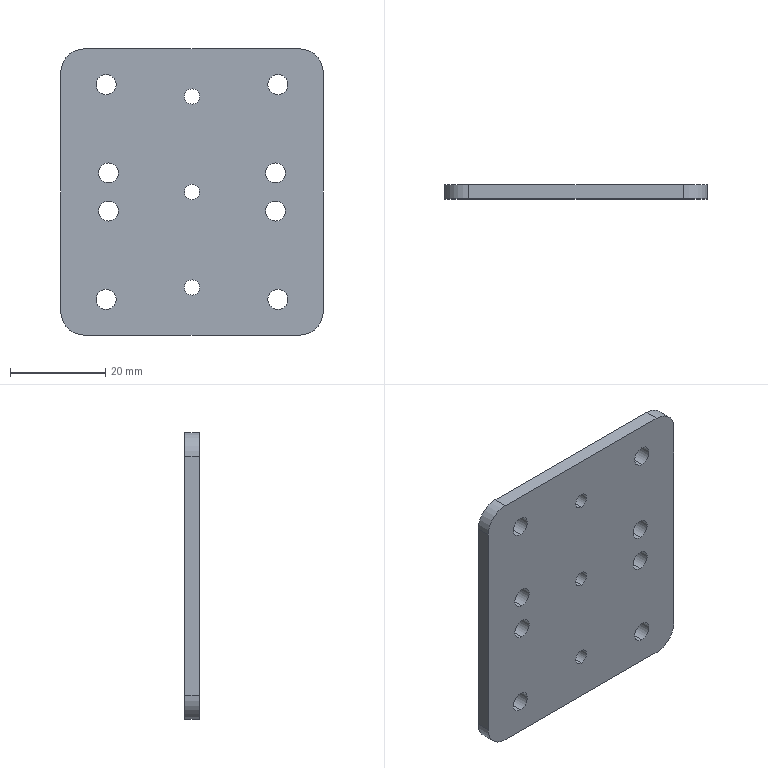Part | SolidWorks | features BaseBody 1 | 1 solid | 32 faces | box 55 x 3 x 60 mm | volume 9431 mm3 | cylinder 26 | plane 6 | commonest cylinder face diameters 4.2 x16 3.2 x6 10 x4
STEP:
#1=CARTESIAN_POINT('',(0.,0.,-21.6));
#2=VERTEX_POINT('',#1);
#3=CARTESIAN_POINT('',(0.,0.,-18.4));
#4=VERTEX_POINT('',#3);
#5=CARTESIAN_POINT('',(0.,0.,-20.));
#6=DIRECTION('',(0.,1.,0.));
#7=DIRECTION('',(0.,0.,1.));
#8=AXIS2_PLACEMENT_3D('',#5,#6,#7);
#9=CIRCLE('',#8,1.6);
#10=EDGE_CURVE('',#2,#4,#9,.T.);
#11=ORIENTED_EDGE('',*,*,#10,.F.);
#12=CARTESIAN_POINT('',(0.,3.,-21.6));
#13=VERTEX_POINT('',#12);
#14=CARTESIAN_POINT('',(0.,0.,-21.6));
#15=DIRECTION('',(0.,1.,0.));
#16=VECTOR('',#15,1000.);
#17=LINE('',#14,#16);
#18=EDGE_CURVE('',#2,#13,#17,.T.);
#19=ORIENTED_EDGE('',*,*,#18,.T.);
#20=CARTESIAN_POINT('',(0.,3.,-18.4));
#21=VERTEX_POINT('',#20);
#22=CARTESIAN_POINT('',(0.,3.,-20.));
#23=DIRECTION('',(0.,1.,0.));
#24=DIRECTION('',(0.,0.,1.));
#25=AXIS2_PLACEMENT_3D('',#22,#23,#24);
#26=CIRCLE('',#25,1.6);
#27=EDGE_CURVE('',#13,#21,#26,.T.);
#28=ORIENTED_EDGE('',*,*,#27,.T.);
#29=CARTESIAN_POINT('',(0.,0.,-18.4));
#30=DIRECTION('',(0.,1.,0.));
#31=VECTOR('',#30,1000.);
#32=LINE('',#29,#31);
#33=EDGE_CURVE('',#4,#21,#32,.T.);
#34=ORIENTED_EDGE('',*,*,#33,.F.);
#35=EDGE_LOOP('',(#11,#19,#28,#34));
#36=FACE_OUTER_BOUND('',#35,.T.);
#37=CARTESIAN_POINT('',(0.,0.,-20.));
#38=DIRECTION('',(0.,1.,0.));
#39=DIRECTION('',(0.,0.,1.));
#40=AXIS2_PLACEMENT_3D('',#37,#38,#39);
#41=CYLINDRICAL_SURFACE('',#40,1.6);
#42=ADVANCED_FACE('',(#36),#41,.F.);
#43=CARTESIAN_POINT('',(0.,0.,18.4));
#44=VERTEX_POINT('',#43);
#45=CARTESIAN_POINT('',(0.,0.,21.6));
#46=VERTEX_POINT('',#45);
#47=CARTESIAN_POINT('',(0.,0.,20.));
#48=DIRECTION('',(0.,1.,0.));
#49=DIRECTION('',(0.,0.,1.));
#50=AXIS2_PLACEMENT_3D('',#47,#48,#49);
#51=CIRCLE('',#50,1.6);
#52=EDGE_CURVE('',#44,#46,#51,.T.);
#53=ORIENTED_EDGE('',*,*,#52,.F.);
#54=CARTESIAN_POINT('',(0.,3.,18.4));
#55=VERTEX_POINT('',#54);
#56=CARTESIAN_POINT('',(0.,0.,18.4));
#57=DIRECTION('',(0.,1.,0.));
#58=VECTOR('',#57,1000.);
#59=LINE('',#56,#58);
#60=EDGE_CURVE('',#44,#55,#59,.T.);
#61=ORIENTED_EDGE('',*,*,#60,.T.);
#62=CARTESIAN_POINT('',(0.,3.,21.6));
#63=VERTEX_POINT('',#62);
#64=CARTESIAN_POINT('',(0.,3.,20.));
#65=DIRECTION('',(0.,1.,0.));
#66=DIRECTION('',(0.,0.,1.));
#67=AXIS2_PLACEMENT_3D('',#64,#65,#66);
#68=CIRCLE('',#67,1.6);
#69=EDGE_CURVE('',#55,#63,#68,.T.);
#70=ORIENTED_EDGE('',*,*,#69,.T.);
#71=CARTESIAN_POINT('',(0.,0.,21.6));
#72=DIRECTION('',(0.,1.,0.));
#73=VECTOR('',#72,1000.);
#74=LINE('',#71,#73);
#75=EDGE_CURVE('',#46,#63,#74,.T.);
#76=ORIENTED_EDGE('',*,*,#75,.F.);
#77=EDGE_LOOP('',(#53,#61,#70,#76));
#78=FACE_OUTER_BOUND('',#77,.T.);
#79=CARTESIAN_POINT('',(0.,0.,20.));
#80=DIRECTION('',(0.,1.,0.));
#81=DIRECTION('',(0.,0.,1.));
#82=AXIS2_PLACEMENT_3D('',#79,#80,#81);
#83=CYLINDRICAL_SURFACE('',#82,1.6);
#84=ADVANCED_FACE('',(#78),#83,.F.);
#85=CARTESIAN_POINT('',(0.,0.,-1.6));
#86=VERTEX_POINT('',#85);
#87=CARTESIAN_POINT('',(0.,0.,1.6));
#88=VERTEX_POINT('',#87);
#89=CARTESIAN_POINT('',(0.,0.,0.));
#90=DIRECTION('',(0.,1.,0.));
#91=DIRECTION('',(0.,0.,1.));
#92=AXIS2_PLACEMENT_3D('',#89,#90,#91);
#93=CIRCLE('',#92,1.6);
#94=EDGE_CURVE('',#86,#88,#93,.T.);
#95=ORIENTED_EDGE('',*,*,#94,.F.);
#96=CARTESIAN_POINT('',(0.,3.,-1.6));
#97=VERTEX_POINT('',#96);
#98=CARTESIAN_POINT('',(0.,0.,-1.6));
#99=DIRECTION('',(0.,1.,0.));
#100=VECTOR('',#99,1000.);
#101=LINE('',#98,#100);
#102=EDGE_CURVE('',#86,#97,#101,.T.);
#103=ORIENTED_EDGE('',*,*,#102,.T.);
#104=CARTESIAN_POINT('',(0.,3.,1.6));
#105=VERTEX_POINT('',#104);
#106=CARTESIAN_POINT('',(0.,3.,0.));
#107=DIRECTION('',(0.,1.,0.));
#108=DIRECTION('',(0.,0.,1.));
#109=AXIS2_PLACEMENT_3D('',#106,#107,#108);
#110=CIRCLE('',#109,1.6);
#111=EDGE_CURVE('',#97,#105,#110,.T.);
#112=ORIENTED_EDGE('',*,*,#111,.T.);
#113=CARTESIAN_POINT('',(0.,0.,1.6));
#114=DIRECTION('',(0.,1.,0.));
#115=VECTOR('',#114,1000.);
#116=LINE('',#113,#115);
#117=EDGE_CURVE('',#88,#105,#116,.T.);
#118=ORIENTED_EDGE('',*,*,#117,.F.);
#119=EDGE_LOOP('',(#95,#103,#112,#118));
#120=FACE_OUTER_BOUND('',#119,.T.);
#121=CARTESIAN_POINT('',(0.,0.,0.));
#122=DIRECTION('',(0.,1.,0.));
#123=DIRECTION('',(0.,0.,1.));
#124=AXIS2_PLACEMENT_3D('',#121,#122,#123);
#125=CYLINDRICAL_SURFACE('',#124,1.6);
#126=ADVANCED_FACE('',(#120),#125,.F.);
#127=CARTESIAN_POINT('',(-18.,0.,-24.6));
#128=VERTEX_POINT('',#127);
#129=CARTESIAN_POINT('',(-18.,0.,-20.4));
#130=VERTEX_POINT('',#129);
#131=CARTESIAN_POINT('',(-18.,0.,-22.5));
#132=DIRECTION('',(0.,1.,0.));
#133=DIRECTION('',(0.,0.,1.));
#134=AXIS2_PLACEMENT_3D('',#131,#132,#133);
#135=CIRCLE('',#134,2.1);
#136=EDGE_CURVE('',#128,#130,#135,.T.);
#137=ORIENTED_EDGE('',*,*,#136,.F.);
#138=CARTESIAN_POINT('',(-18.,3.,-24.6));
#139=VERTEX_POINT('',#138);
#140=CARTESIAN_POINT('',(-18.,0.,-24.6));
#141=DIRECTION('',(0.,1.,0.));
#142=VECTOR('',#141,1000.);
#143=LINE('',#140,#142);
#144=EDGE_CURVE('',#128,#139,#143,.T.);
#145=ORIENTED_EDGE('',*,*,#144,.T.);
#146=CARTESIAN_POINT('',(-18.,3.,-20.4));
#147=VERTEX_POINT('',#146);
#148=CARTESIAN_POINT('',(-18.,3.,-22.5));
#149=DIRECTION('',(0.,1.,0.));
#150=DIRECTION('',(0.,0.,1.));
#151=AXIS2_PLACEMENT_3D('',#148,#149,#150);
#152=CIRCLE('',#151,2.1);
#153=EDGE_CURVE('',#139,#147,#152,.T.);
#154=ORIENTED_EDGE('',*,*,#153,.T.);
#155=CARTESIAN_POINT('',(-18.,0.,-20.4));
#156=DIRECTION('',(0.,1.,0.));
#157=VECTOR('',#156,1000.);
#158=LINE('',#155,#157);
#159=EDGE_CURVE('',#130,#147,#158,.T.);
#160=ORIENTED_EDGE('',*,*,#159,.F.);
#161=EDGE_LOOP('',(#137,#145,#154,#160));
#162=FACE_OUTER_BOUND('',#161,.T.);
#163=CARTESIAN_POINT('',(-18.,0.,-22.5));
#164=DIRECTION('',(0.,1.,0.));
#165=DIRECTION('',(0.,0.,1.));
#166=AXIS2_PLACEMENT_3D('',#163,#164,#165);
#167=CYLINDRICAL_SURFACE('',#166,2.1);
#168=ADVANCED_FACE('',(#162),#167,.F.);
#169=CARTESIAN_POINT('',(-18.,0.,20.4));
#170=VERTEX_POINT('',#169);
#171=CARTESIAN_POINT('',(-18.,0.,24.6));
#172=VERTEX_POINT('',#171);
#173=CARTESIAN_POINT('',(-18.,0.,22.5));
#174=DIRECTION('',(0.,1.,0.));
#175=DIRECTION('',(0.,0.,1.));
#176=AXIS2_PLACEMENT_3D('',#173,#174,#175);
#177=CIRCLE('',#176,2.1);
#178=EDGE_CURVE('',#170,#172,#177,.T.);
#179=ORIENTED_EDGE('',*,*,#178,.F.);
#180=CARTESIAN_POINT('',(-18.,3.,20.4));
#181=VERTEX_POINT('',#180);
#182=CARTESIAN_POINT('',(-18.,0.,20.4));
#183=DIRECTION('',(0.,1.,0.));
#184=VECTOR('',#183,1000.);
#185=LINE('',#182,#184);
#186=EDGE_CURVE('',#170,#181,#185,.T.);
#187=ORIENTED_EDGE('',*,*,#186,.T.);
#188=CARTESIAN_POINT('',(-18.,3.,24.6));
#189=VERTEX_POINT('',#188);
#190=CARTESIAN_POINT('',(-18.,3.,22.5));
#191=DIRECTION('',(0.,1.,0.));
#192=DIRECTION('',(0.,0.,1.));
#193=AXIS2_PLACEMENT_3D('',#190,#191,#192);
#194=CIRCLE('',#193,2.1);
#195=EDGE_CURVE('',#181,#189,#194,.T.);
#196=ORIENTED_EDGE('',*,*,#195,.T.);
#197=CARTESIAN_POINT('',(-18.,0.,24.6));
#198=DIRECTION('',(0.,1.,0.));
#199=VECTOR('',#198,1000.);
#200=LINE('',#197,#199);
#201=EDGE_CURVE('',#172,#189,#200,.T.);
#202=ORIENTED_EDGE('',*,*,#201,.F.);
#203=EDGE_LOOP('',(#179,#187,#196,#202));
#204=FACE_OUTER_BOUND('',#203,.T.);
#205=CARTESIAN_POINT('',(-18.,0.,22.5));
#206=DIRECTION('',(0.,1.,0.));
#207=DIRECTION('',(0.,0.,1.));
#208=AXIS2_PLACEMENT_3D('',#205,#206,#207);
#209=CYLINDRICAL_SURFACE('',#208,2.1);
#210=ADVANCED_FACE('',(#204),#209,.F.);
#211=CARTESIAN_POINT('',(18.,0.,20.4));
#212=VERTEX_POINT('',#211);
#213=CARTESIAN_POINT('',(18.,0.,24.6));
#214=VERTEX_POINT('',#213);
#215=CARTESIAN_POINT('',(18.,0.,22.5));
#216=DIRECTION('',(0.,1.,0.));
#217=DIRECTION('',(0.,0.,1.));
#218=AXIS2_PLACEMENT_3D('',#215,#216,#217);
#219=CIRCLE('',#218,2.1);
#220=EDGE_CURVE('',#212,#214,#219,.T.);
#221=ORIENTED_EDGE('',*,*,#220,.F.);
#222=CARTESIAN_POINT('',(18.,3.,20.4));
#223=VERTEX_POINT('',#222);
#224=CARTESIAN_POINT('',(18.,0.,20.4));
#225=DIRECTION('',(0.,1.,0.));
#226=VECTOR('',#225,1000.);
#227=LINE('',#224,#226);
#228=EDGE_CURVE('',#212,#223,#227,.T.);
#229=ORIENTED_EDGE('',*,*,#228,.T.);
#230=CARTESIAN_POINT('',(18.,3.,24.6));
#231=VERTEX_POINT('',#230);
#232=CARTESIAN_POINT('',(18.,3.,22.5));
#233=DIRECTION('',(0.,1.,0.));
#234=DIRECTION('',(0.,0.,1.));
#235=AXIS2_PLACEMENT_3D('',#232,#233,#234);
#236=CIRCLE('',#235,2.1);
#237=EDGE_CURVE('',#223,#231,#236,.T.);
#238=ORIENTED_EDGE('',*,*,#237,.T.);
#239=CARTESIAN_POINT('',(18.,0.,24.6));
#240=DIRECTION('',(0.,1.,0.));
#241=VECTOR('',#240,1000.);
#242=LINE('',#239,#241);
#243=EDGE_CURVE('',#214,#231,#242,.T.);
#244=ORIENTED_EDGE('',*,*,#243,.F.);
#245=EDGE_LOOP('',(#221,#229,#238,#244));
#246=FACE_OUTER_BOUND('',#245,.T.);
#247=CARTESIAN_POINT('',(18.,0.,22.5));
#248=DIRECTION('',(0.,1.,0.));
#249=DIRECTION('',(0.,0.,1.));
#250=AXIS2_PLACEMENT_3D('',#247,#248,#249);
#251=CYLINDRICAL_SURFACE('',#250,2.1);
#252=ADVANCED_FACE('',(#246),#251,.F.);
#253=CARTESIAN_POINT('',(18.,0.,-24.6));
#254=VERTEX_POINT('',#253);
#255=CARTESIAN_POINT('',(18.,0.,-20.4));
#256=VERTEX_POINT('',#255);
#257=CARTESIAN_POINT('',(18.,0.,-22.5));
#258=DIRECTION('',(0.,1.,0.));
#259=DIRECTION('',(0.,0.,1.));
#260=AXIS2_PLACEMENT_3D('',#257,#258,#259);
#261=CIRCLE('',#260,2.1);
#262=EDGE_CURVE('',#254,#256,#261,.T.);
#263=ORIENTED_EDGE('',*,*,#262,.F.);
#264=CARTESIAN_POINT('',(18.,3.,-24.6));
#265=VERTEX_POINT('',#264);
#266=CARTESIAN_POINT('',(18.,0.,-24.6));
#267=DIRECTION('',(0.,1.,0.));
#268=VECTOR('',#267,1000.);
#269=LINE('',#266,#268);
#270=EDGE_CURVE('',#254,#265,#269,.T.);
#271=ORIENTED_EDGE('',*,*,#270,.T.);
#272=CARTESIAN_POINT('',(18.,3.,-20.4));
#273=VERTEX_POINT('',#272);
#274=CARTESIAN_POINT('',(18.,3.,-22.5));
#275=DIRECTION('',(0.,1.,0.));
#276=DIRECTION('',(0.,0.,1.));
#277=AXIS2_PLACEMENT_3D('',#274,#275,#276);
#278=CIRCLE('',#277,2.1);
#279=EDGE_CURVE('',#265,#273,#278,.T.);
#280=ORIENTED_EDGE('',*,*,#279,.T.);
#281=CARTESIAN_POINT('',(18.,0.,-20.4));
#282=DIRECTION('',(0.,1.,0.));
#283=VECTOR('',#282,1000.);
#284=LINE('',#281,#283);
#285=EDGE_CURVE('',#256,#273,#284,.T.);
#286=ORIENTED_EDGE('',*,*,#285,.F.);
#287=EDGE_LOOP('',(#263,#271,#280,#286));
#288=FACE_OUTER_BOUND('',#287,.T.);
#289=CARTESIAN_POINT('',(18.,0.,-22.5));
#290=DIRECTION('',(0.,1.,0.));
#291=DIRECTION('',(0.,0.,1.));
#292=AXIS2_PLACEMENT_3D('',#289,#290,#291);
#293=CYLINDRICAL_SURFACE('',#292,2.1);
#294=ADVANCED_FACE('',(#288),#293,.F.);
#295=CARTESIAN_POINT('',(17.5,0.,-6.1));
#296=VERTEX_POINT('',#295);
#297=CARTESIAN_POINT('',(17.5,0.,-1.9));
#298=VERTEX_POINT('',#297);
#299=CARTESIAN_POINT('',(17.5,0.,-4.));
#300=DIRECTION('',(0.,1.,0.));
#301=DIRECTION('',(0.,0.,1.));
#302=AXIS2_PLACEMENT_3D('',#299,#300,#301);
#303=CIRCLE('',#302,2.1);
#304=EDGE_CURVE('',#296,#298,#303,.T.);
#305=ORIENTED_EDGE('',*,*,#304,.F.);
#306=CARTESIAN_POINT('',(17.5,3.,-6.1));
#307=VERTEX_POINT('',#306);
#308=CARTESIAN_POINT('',(17.5,0.,-6.1));
#309=DIRECTION('',(0.,1.,0.));
#310=VECTOR('',#309,1000.);
#311=LINE('',#308,#310);
#312=EDGE_CURVE('',#296,#307,#311,.T.);
#313=ORIENTED_EDGE('',*,*,#312,.T.);
#314=CARTESIAN_POINT('',(17.5,3.,-1.9));
#315=VERTEX_POINT('',#314);
#316=CARTESIAN_POINT('',(17.5,3.,-4.));
#317=DIRECTION('',(0.,1.,0.));
#318=DIRECTION('',(0.,0.,1.));
#319=AXIS2_PLACEMENT_3D('',#316,#317,#318);
#320=CIRCLE('',#319,2.1);
#321=EDGE_CURVE('',#307,#315,#320,.T.);
#322=ORIENTED_EDGE('',*,*,#321,.T.);
#323=CARTESIAN_POINT('',(17.5,0.,-1.9));
#324=DIRECTION('',(0.,1.,0.));
#325=VECTOR('',#324,1000.);
#326=LINE('',#323,#325);
#327=EDGE_CURVE('',#298,#315,#326,.T.);
#328=ORIENTED_EDGE('',*,*,#327,.F.);
#329=EDGE_LOOP('',(#305,#313,#322,#328));
#330=FACE_OUTER_BOUND('',#329,.T.);
#331=CARTESIAN_POINT('',(17.5,0.,-4.));
#332=DIRECTION('',(0.,1.,0.));
#333=DIRECTION('',(0.,0.,1.));
#334=AXIS2_PLACEMENT_3D('',#331,#332,#333);
#335=CYLINDRICAL_SURFACE('',#334,2.1);
#336=ADVANCED_FACE('',(#330),#335,.F.);
#337=CARTESIAN_POINT('',(-17.5,0.,1.9));
#338=VERTEX_POINT('',#337);
#339=CARTESIAN_POINT('',(-17.5,0.,6.1));
#340=VERTEX_POINT('',#339);
#341=CARTESIAN_POINT('',(-17.5,0.,4.));
#342=DIRECTION('',(0.,1.,0.));
#343=DIRECTION('',(0.,0.,1.));
#344=AXIS2_PLACEMENT_3D('',#341,#342,#343);
#345=CIRCLE('',#344,2.1);
#346=EDGE_CURVE('',#338,#340,#345,.T.);
#347=ORIENTED_EDGE('',*,*,#346,.F.);
#348=CARTESIAN_POINT('',(-17.5,3.,1.9));
#349=VERTEX_POINT('',#348);
#350=CARTESIAN_POINT('',(-17.5,0.,1.9));
#351=DIRECTION('',(0.,1.,0.));
#352=VECTOR('',#351,1000.);
#353=LINE('',#350,#352);
#354=EDGE_CURVE('',#338,#349,#353,.T.);
#355=ORIENTED_EDGE('',*,*,#354,.T.);
#356=CARTESIAN_POINT('',(-17.5,3.,6.1));
#357=VERTEX_POINT('',#356);
#358=CARTESIAN_POINT('',(-17.5,3.,4.));
#359=DIRECTION('',(0.,1.,0.));
#360=DIRECTION('',(0.,0.,1.));
#361=AXIS2_PLACEMENT_3D('',#358,#359,#360);
#362=CIRCLE('',#361,2.1);
#363=EDGE_CURVE('',#349,#357,#362,.T.);
#364=ORIENTED_EDGE('',*,*,#363,.T.);
#365=CARTESIAN_POINT('',(-17.5,0.,6.1));
#366=DIRECTION('',(0.,1.,0.));
#367=VECTOR('',#366,1000.);
#368=LINE('',#365,#367);
#369=EDGE_CURVE('',#340,#357,#368,.T.);
#370=ORIENTED_EDGE('',*,*,#369,.F.);
#371=EDGE_LOOP('',(#347,#355,#364,#370));
#372=FACE_OUTER_BOUND('',#371,.T.);
#373=CARTESIAN_POINT('',(-17.5,0.,4.));
#374=DIRECTION('',(0.,1.,0.));
#375=DIRECTION('',(0.,0.,1.));
#376=AXIS2_PLACEMENT_3D('',#373,#374,#375);
#377=CYLINDRICAL_SURFACE('',#376,2.1);
#378=ADVANCED_FACE('',(#372),#377,.F.);
#379=CARTESIAN_POINT('',(-17.5,0.,-6.1));
#380=VERTEX_POINT('',#379);
#381=CARTESIAN_POINT('',(-17.5,0.,-1.9));
#382=VERTEX_POINT('',#381);
#383=CARTESIAN_POINT('',(-17.5,0.,-4.));
#384=DIRECTION('',(0.,1.,0.));
#385=DIRECTION('',(0.,0.,1.));
#386=AXIS2_PLACEMENT_3D('',#383,#384,#385);
#387=CIRCLE('',#386,2.1);
#388=EDGE_CURVE('',#380,#382,#387,.T.);
#389=ORIENTED_EDGE('',*,*,#388,.F.);
#390=CARTESIAN_POINT('',(-17.5,3.,-6.1));
#391=VERTEX_POINT('',#390);
#392=CARTESIAN_POINT('',(-17.5,0.,-6.1));
#393=DIRECTION('',(0.,1.,0.));
#394=VECTOR('',#393,1000.);
#395=LINE('',#392,#394);
#396=EDGE_CURVE('',#380,#391,#395,.T.);
#397=ORIENTED_EDGE('',*,*,#396,.T.);
#398=CARTESIAN_POINT('',(-17.5,3.,-1.9));
#399=VERTEX_POINT('',#398);
#400=CARTESIAN_POINT('',(-17.5,3.,-4.));
#401=DIRECTION('',(0.,1.,0.));
#402=DIRECTION('',(0.,0.,1.));
#403=AXIS2_PLACEMENT_3D('',#400,#401,#402);
#404=CIRCLE('',#403,2.1);
#405=EDGE_CURVE('',#391,#399,#404,.T.);
#406=ORIENTED_EDGE('',*,*,#405,.T.);
#407=CARTESIAN_POINT('',(-17.5,0.,-1.9));
#408=DIRECTION('',(0.,1.,0.));
#409=VECTOR('',#408,1000.);
#410=LINE('',#407,#409);
#411=EDGE_CURVE('',#382,#399,#410,.T.);
#412=ORIENTED_EDGE('',*,*,#411,.F.);
#413=EDGE_LOOP('',(#389,#397,#406,#412));
#414=FACE_OUTER_BOUND('',#413,.T.);
#415=CARTESIAN_POINT('',(-17.5,0.,-4.));
#416=DIRECTION('',(0.,1.,0.));
#417=DIRECTION('',(0.,0.,1.));
#418=AXIS2_PLACEMENT_3D('',#415,#416,#417);
#419=CYLINDRICAL_SURFACE('',#418,2.1);
#420=ADVANCED_FACE('',(#414),#419,.F.);
#421=CARTESIAN_POINT('',(17.5,0.,1.9));
#422=VERTEX_POINT('',#421);
#423=CARTESIAN_POINT('',(17.5,0.,6.1));
#424=VERTEX_POINT('',#423);
#425=CARTESIAN_POINT('',(17.5,0.,4.));
#426=DIRECTION('',(0.,1.,0.));
#427=DIRECTION('',(0.,0.,1.));
#428=AXIS2_PLACEMENT_3D('',#425,#426,#427);
#429=CIRCLE('',#428,2.1);
#430=EDGE_CURVE('',#422,#424,#429,.T.);
#431=ORIENTED_EDGE('',*,*,#430,.F.);
#432=CARTESIAN_POINT('',(17.5,3.,1.9));
#433=VERTEX_POINT('',#432);
#434=CARTESIAN_POINT('',(17.5,0.,1.9));
#435=DIRECTION('',(0.,1.,0.));
#436=VECTOR('',#435,1000.);
#437=LINE('',#434,#436);
#438=EDGE_CURVE('',#422,#433,#437,.T.);
#439=ORIENTED_EDGE('',*,*,#438,.T.);
#440=CARTESIAN_POINT('',(17.5,3.,6.1));
#441=VERTEX_POINT('',#440);
#442=CARTESIAN_POINT('',(17.5,3.,4.));
#443=DIRECTION('',(0.,1.,0.));
#444=DIRECTION('',(0.,0.,1.));
#445=AXIS2_PLACEMENT_3D('',#442,#443,#444);
#446=CIRCLE('',#445,2.1);
#447=EDGE_CURVE('',#433,#441,#446,.T.);
#448=ORIENTED_EDGE('',*,*,#447,.T.);
#449=CARTESIAN_POINT('',(17.5,0.,6.1));
#450=DIRECTION('',(0.,1.,0.));
#451=VECTOR('',#450,1000.);
#452=LINE('',#449,#451);
#453=EDGE_CURVE('',#424,#441,#452,.T.);
#454=ORIENTED_EDGE('',*,*,#453,.F.);
#455=EDGE_LOOP('',(#431,#439,#448,#454));
#456=FACE_OUTER_BOUND('',#455,.T.);
#457=CARTESIAN_POINT('',(17.5,0.,4.));
#458=DIRECTION('',(0.,1.,0.));
#459=DIRECTION('',(0.,0.,1.));
#460=AXIS2_PLACEMENT_3D('',#457,#458,#459);
#461=CYLINDRICAL_SURFACE('',#460,2.1);
#462=ADVANCED_FACE('',(#456),#461,.F.);
#463=CARTESIAN_POINT('',(-27.5,3.,-25.));
#464=VERTEX_POINT('',#463);
#465=CARTESIAN_POINT('',(-22.5,3.,-30.));
#466=VERTEX_POINT('',#465);
#467=CARTESIAN_POINT('',(-22.5,3.,-25.));
#468=DIRECTION('',(0.,-1.,0.));
#469=DIRECTION('',(0.,0.,-1.));
#470=AXIS2_PLACEMENT_3D('',#467,#468,#469);
#471=CIRCLE('',#470,5.);
#472=EDGE_CURVE('',#464,#466,#471,.T.);
#473=ORIENTED_EDGE('',*,*,#472,.F.);
#474=CARTESIAN_POINT('',(-27.5,3.,25.));
#475=VERTEX_POINT('',#474);
#476=CARTESIAN_POINT('',(-27.5,3.,0.));
#477=DIRECTION('',(0.,0.,-1.));
#478=VECTOR('',#477,1000.);
#479=LINE('',#476,#478);
#480=EDGE_CURVE('',#475,#464,#479,.T.);
#481=ORIENTED_EDGE('',*,*,#480,.F.);
#482=CARTESIAN_POINT('',(-22.5,3.,30.));
#483=VERTEX_POINT('',#482);
#484=CARTESIAN_POINT('',(-22.5,3.,25.));
#485=DIRECTION('',(0.,-1.,0.));
#486=DIRECTION('',(0.,0.,-1.));
#487=AXIS2_PLACEMENT_3D('',#484,#485,#486);
#488=CIRCLE('',#487,5.);
#489=EDGE_CURVE('',#483,#475,#488,.T.);
#490=ORIENTED_EDGE('',*,*,#489,.F.);
#491=CARTESIAN_POINT('',(22.5,3.,30.));
#492=VERTEX_POINT('',#491);
#493=CARTESIAN_POINT('',(0.,3.,30.));
#494=DIRECTION('',(-1.,0.,0.));
#495=VECTOR('',#494,1000.);
#496=LINE('',#493,#495);
#497=EDGE_CURVE('',#492,#483,#496,.T.);
#498=ORIENTED_EDGE('',*,*,#497,.F.);
#499=CARTESIAN_POINT('',(27.5,3.,25.));
#500=VERTEX_POINT('',#499);
#501=CARTESIAN_POINT('',(22.5,3.,25.));
#502=DIRECTION('',(0.,-1.,0.));
#503=DIRECTION('',(0.,0.,-1.));
#504=AXIS2_PLACEMENT_3D('',#501,#502,#503);
#505=CIRCLE('',#504,5.);
#506=EDGE_CURVE('',#500,#492,#505,.T.);
#507=ORIENTED_EDGE('',*,*,#506,.F.);
#508=CARTESIAN_POINT('',(27.5,3.,-25.));
#509=VERTEX_POINT('',#508);
#510=CARTESIAN_POINT('',(27.5,3.,0.));
#511=DIRECTION('',(0.,0.,1.));
#512=VECTOR('',#511,1000.);
#513=LINE('',#510,#512);
#514=EDGE_CURVE('',#509,#500,#513,.T.);
#515=ORIENTED_EDGE('',*,*,#514,.F.);
#516=CARTESIAN_POINT('',(22.5,3.,-30.));
#517=VERTEX_POINT('',#516);
#518=CARTESIAN_POINT('',(22.5,3.,-25.));
#519=DIRECTION('',(0.,-1.,0.));
#520=DIRECTION('',(0.,0.,-1.));
#521=AXIS2_PLACEMENT_3D('',#518,#519,#520);
#522=CIRCLE('',#521,5.);
#523=EDGE_CURVE('',#517,#509,#522,.T.);
#524=ORIENTED_EDGE('',*,*,#523,.F.);
#525=CARTESIAN_POINT('',(0.,3.,-30.));
#526=DIRECTION('',(1.,0.,0.));
#527=VECTOR('',#526,1000.);
#528=LINE('',#525,#527);
#529=EDGE_CURVE('',#466,#517,#528,.T.);
#530=ORIENTED_EDGE('',*,*,#529,.F.);
#531=EDGE_LOOP('',(#473,#481,#490,#498,#507,#515,#524,#530));
#532=FACE_OUTER_BOUND('',#531,.T.);
#533=CARTESIAN_POINT('',(0.,3.,-20.));
#534=DIRECTION('',(0.,1.,0.));
#535=DIRECTION('',(0.,0.,1.));
#536=AXIS2_PLACEMENT_3D('',#533,#534,#535);
#537=CIRCLE('',#536,1.6);
#538=EDGE_CURVE('',#21,#13,#537,.T.);
#539=ORIENTED_EDGE('',*,*,#538,.F.);
#540=ORIENTED_EDGE('',*,*,#27,.F.);
#541=EDGE_LOOP('',(#539,#540));
#542=FACE_BOUND('',#541,.T.);
#543=CARTESIAN_POINT('',(0.,3.,20.));
#544=DIRECTION('',(0.,1.,0.));
#545=DIRECTION('',(0.,0.,1.));
#546=AXIS2_PLACEMENT_3D('',#543,#544,#545);
#547=CIRCLE('',#546,1.6);
#548=EDGE_CURVE('',#63,#55,#547,.T.);
#549=ORIENTED_EDGE('',*,*,#548,.F.);
#550=ORIENTED_EDGE('',*,*,#69,.F.);
#551=EDGE_LOOP('',(#549,#550));
#552=FACE_BOUND('',#551,.T.);
#553=CARTESIAN_POINT('',(0.,3.,0.));
#554=DIRECTION('',(0.,1.,0.));
#555=DIRECTION('',(0.,0.,1.));
#556=AXIS2_PLACEMENT_3D('',#553,#554,#555);
#557=CIRCLE('',#556,1.6);
#558=EDGE_CURVE('',#105,#97,#557,.T.);
#559=ORIENTED_EDGE('',*,*,#558,.F.);
#560=ORIENTED_EDGE('',*,*,#111,.F.);
#561=EDGE_LOOP('',(#559,#560));
#562=FACE_BOUND('',#561,.T.);
#563=CARTESIAN_POINT('',(-18.,3.,-22.5));
#564=DIRECTION('',(0.,1.,0.));
#565=DIRECTION('',(0.,0.,1.));
#566=AXIS2_PLACEMENT_3D('',#563,#564,#565);
#567=CIRCLE('',#566,2.1);
#568=EDGE_CURVE('',#147,#139,#567,.T.);
#569=ORIENTED_EDGE('',*,*,#568,.F.);
#570=ORIENTED_EDGE('',*,*,#153,.F.);
#571=EDGE_LOOP('',(#569,#570));
#572=FACE_BOUND('',#571,.T.);
#573=CARTESIAN_POINT('',(-18.,3.,22.5));
#574=DIRECTION('',(0.,1.,0.));
#575=DIRECTION('',(0.,0.,1.));
#576=AXIS2_PLACEMENT_3D('',#573,#574,#575);
#577=CIRCLE('',#576,2.1);
#578=EDGE_CURVE('',#189,#181,#577,.T.);
#579=ORIENTED_EDGE('',*,*,#578,.F.);
#580=ORIENTED_EDGE('',*,*,#195,.F.);
#581=EDGE_LOOP('',(#579,#580));
#582=FACE_BOUND('',#581,.T.);
#583=CARTESIAN_POINT('',(18.,3.,22.5));
#584=DIRECTION('',(0.,1.,0.));
#585=DIRECTION('',(0.,0.,1.));
#586=AXIS2_PLACEMENT_3D('',#583,#584,#585);
#587=CIRCLE('',#586,2.1);
#588=EDGE_CURVE('',#231,#223,#587,.T.);
#589=ORIENTED_EDGE('',*,*,#588,.F.);
#590=ORIENTED_EDGE('',*,*,#237,.F.);
#591=EDGE_LOOP('',(#589,#590));
#592=FACE_BOUND('',#591,.T.);
#593=CARTESIAN_POINT('',(18.,3.,-22.5));
#594=DIRECTION('',(0.,1.,0.));
#595=DIRECTION('',(0.,0.,1.));
#596=AXIS2_PLACEMENT_3D('',#593,#594,#595);
#597=CIRCLE('',#596,2.1);
#598=EDGE_CURVE('',#273,#265,#597,.T.);
#599=ORIENTED_EDGE('',*,*,#598,.F.);
#600=ORIENTED_EDGE('',*,*,#279,.F.);
#601=EDGE_LOOP('',(#599,#600));
#602=FACE_BOUND('',#601,.T.);
#603=CARTESIAN_POINT('',(17.5,3.,-4.));
#604=DIRECTION('',(0.,1.,0.));
#605=DIRECTION('',(0.,0.,1.));
#606=AXIS2_PLACEMENT_3D('',#603,#604,#605);
#607=CIRCLE('',#606,2.1);
#608=EDGE_CURVE('',#315,#307,#607,.T.);
#609=ORIENTED_EDGE('',*,*,#608,.F.);
#610=ORIENTED_EDGE('',*,*,#321,.F.);
#611=EDGE_LOOP('',(#609,#610));
#612=FACE_BOUND('',#611,.T.);
#613=CARTESIAN_POINT('',(-17.5,3.,4.));
#614=DIRECTION('',(0.,1.,0.));
#615=DIRECTION('',(0.,0.,1.));
#616=AXIS2_PLACEMENT_3D('',#613,#614,#615);
#617=CIRCLE('',#616,2.1);
#618=EDGE_CURVE('',#357,#349,#617,.T.);
#619=ORIENTED_EDGE('',*,*,#618,.F.);
#620=ORIENTED_EDGE('',*,*,#363,.F.);
#621=EDGE_LOOP('',(#619,#620));
#622=FACE_BOUND('',#621,.T.);
#623=CARTESIAN_POINT('',(-17.5,3.,-4.));
#624=DIRECTION('',(0.,1.,0.));
#625=DIRECTION('',(0.,0.,1.));
#626=AXIS2_PLACEMENT_3D('',#623,#624,#625);
#627=CIRCLE('',#626,2.1);
#628=EDGE_CURVE('',#399,#391,#627,.T.);
#629=ORIENTED_EDGE('',*,*,#628,.F.);
#630=ORIENTED_EDGE('',*,*,#405,.F.);
#631=EDGE_LOOP('',(#629,#630));
#632=FACE_BOUND('',#631,.T.);
#633=CARTESIAN_POINT('',(17.5,3.,4.));
#634=DIRECTION('',(0.,1.,0.));
#635=DIRECTION('',(0.,0.,1.));
#636=AXIS2_PLACEMENT_3D('',#633,#634,#635);
#637=CIRCLE('',#636,2.1);
#638=EDGE_CURVE('',#441,#433,#637,.T.);
#639=ORIENTED_EDGE('',*,*,#638,.F.);
#640=ORIENTED_EDGE('',*,*,#447,.F.);
#641=EDGE_LOOP('',(#639,#640));
#642=FACE_BOUND('',#641,.T.);
#643=CARTESIAN_POINT('',(0.,3.,0.));
#644=DIRECTION('',(0.,-1.,0.));
#645=DIRECTION('',(0.,0.,-1.));
#646=AXIS2_PLACEMENT_3D('',#643,#644,#645);
#647=PLANE('',#646);
#648=ADVANCED_FACE('',(#532,#542,#552,#562,#572,#582,#592,#602,#612,#622,#632,#642),#647,.F.);
#649=CARTESIAN_POINT('',(-22.5,0.,-30.));
#650=VERTEX_POINT('',#649);
#651=CARTESIAN_POINT('',(-22.5,3.,-30.));
#652=DIRECTION('',(0.,-1.,0.));
#653=VECTOR('',#652,1000.);
#654=LINE('',#651,#653);
#655=EDGE_CURVE('',#466,#650,#654,.T.);
#656=ORIENTED_EDGE('',*,*,#655,.F.);
#657=ORIENTED_EDGE('',*,*,#529,.T.);
#658=CARTESIAN_POINT('',(22.5,0.,-30.));
#659=VERTEX_POINT('',#658);
#660=CARTESIAN_POINT('',(22.5,3.,-30.));
#661=DIRECTION('',(0.,1.,0.));
#662=VECTOR('',#661,1000.);
#663=LINE('',#660,#662);
#664=EDGE_CURVE('',#659,#517,#663,.T.);
#665=ORIENTED_EDGE('',*,*,#664,.F.);
#666=CARTESIAN_POINT('',(-120.,0.,-30.));
#667=DIRECTION('',(1.,0.,0.));
#668=VECTOR('',#667,1000.);
#669=LINE('',#666,#668);
#670=EDGE_CURVE('',#650,#659,#669,.T.);
#671=ORIENTED_EDGE('',*,*,#670,.F.);
#672=EDGE_LOOP('',(#656,#657,#665,#671));
#673=FACE_OUTER_BOUND('',#672,.T.);
#674=CARTESIAN_POINT('',(-120.,3.,-30.));
#675=DIRECTION('',(0.,0.,1.));
#676=DIRECTION('',(1.,0.,0.));
#677=AXIS2_PLACEMENT_3D('',#674,#675,#676);
#678=PLANE('',#677);
#679=ADVANCED_FACE('',(#673),#678,.F.);
#680=ORIENTED_EDGE('',*,*,#472,.T.);
#681=ORIENTED_EDGE('',*,*,#655,.T.);
#682=CARTESIAN_POINT('',(-27.5,0.,-25.));
#683=VERTEX_POINT('',#682);
#684=CARTESIAN_POINT('',(-22.5,0.,-25.));
#685=DIRECTION('',(0.,1.,0.));
#686=DIRECTION('',(0.,0.,-1.));
#687=AXIS2_PLACEMENT_3D('',#684,#685,#686);
#688=CIRCLE('',#687,5.);
#689=EDGE_CURVE('',#650,#683,#688,.T.);
#690=ORIENTED_EDGE('',*,*,#689,.T.);
#691=CARTESIAN_POINT('',(-27.5,3.,-25.));
#692=DIRECTION('',(0.,1.,0.));
#693=VECTOR('',#692,1000.);
#694=LINE('',#691,#693);
#695=EDGE_CURVE('',#683,#464,#694,.T.);
#696=ORIENTED_EDGE('',*,*,#695,.T.);
#697=EDGE_LOOP('',(#680,#681,#690,#696));
#698=FACE_OUTER_BOUND('',#697,.T.);
#699=CARTESIAN_POINT('',(-22.5,3.,-25.));
#700=DIRECTION('',(0.,-1.,0.));
#701=DIRECTION('',(0.,0.,-1.));
#702=AXIS2_PLACEMENT_3D('',#699,#700,#701);
#703=CYLINDRICAL_SURFACE('',#702,5.);
#704=ADVANCED_FACE('',(#698),#703,.T.);
#705=CARTESIAN_POINT('',(-27.5,0.,25.));
#706=VERTEX_POINT('',#705);
#707=CARTESIAN_POINT('',(-27.5,0.,30.));
#708=DIRECTION('',(0.,0.,1.));
#709=VECTOR('',#708,1000.);
#710=LINE('',#707,#709);
#711=EDGE_CURVE('',#683,#706,#710,.T.);
#712=ORIENTED_EDGE('',*,*,#711,.T.);
#713=CARTESIAN_POINT('',(-27.5,-7.,25.));
#714=DIRECTION('',(0.,1.,0.));
#715=VECTOR('',#714,1000.);
#716=LINE('',#713,#715);
#717=EDGE_CURVE('',#706,#475,#716,.T.);
#718=ORIENTED_EDGE('',*,*,#717,.T.);
#719=ORIENTED_EDGE('',*,*,#480,.T.);
#720=ORIENTED_EDGE('',*,*,#695,.F.);
#721=EDGE_LOOP('',(#712,#718,#719,#720));
#722=FACE_OUTER_BOUND('',#721,.T.);
#723=CARTESIAN_POINT('',(-27.5,-7.,30.));
#724=DIRECTION('',(-1.,0.,0.));
#725=DIRECTION('',(0.,0.,1.));
#726=AXIS2_PLACEMENT_3D('',#723,#724,#725);
#727=PLANE('',#726);
#728=ADVANCED_FACE('',(#722),#727,.T.);
#729=ORIENTED_EDGE('',*,*,#489,.T.);
#730=ORIENTED_EDGE('',*,*,#717,.F.);
#731=CARTESIAN_POINT('',(-22.5,0.,30.));
#732=VERTEX_POINT('',#731);
#733=CARTESIAN_POINT('',(-22.5,0.,25.));
#734=DIRECTION('',(0.,1.,0.));
#735=DIRECTION('',(0.,0.,-1.));
#736=AXIS2_PLACEMENT_3D('',#733,#734,#735);
#737=CIRCLE('',#736,5.);
#738=EDGE_CURVE('',#706,#732,#737,.T.);
#739=ORIENTED_EDGE('',*,*,#738,.T.);
#740=CARTESIAN_POINT('',(-22.5,-7.,30.));
#741=DIRECTION('',(0.,1.,0.));
#742=VECTOR('',#741,1000.);
#743=LINE('',#740,#742);
#744=EDGE_CURVE('',#732,#483,#743,.T.);
#745=ORIENTED_EDGE('',*,*,#744,.T.);
#746=EDGE_LOOP('',(#729,#730,#739,#745));
#747=FACE_OUTER_BOUND('',#746,.T.);
#748=CARTESIAN_POINT('',(-22.5,-7.,25.));
#749=DIRECTION('',(0.,-1.,0.));
#750=DIRECTION('',(0.,0.,-1.));
#751=AXIS2_PLACEMENT_3D('',#748,#749,#750);
#752=CYLINDRICAL_SURFACE('',#751,5.);
#753=ADVANCED_FACE('',(#747),#752,.T.);
#754=CARTESIAN_POINT('',(22.5,0.,30.));
#755=VERTEX_POINT('',#754);
#756=CARTESIAN_POINT('',(22.5,3.,30.));
#757=DIRECTION('',(0.,-1.,0.));
#758=VECTOR('',#757,1000.);
#759=LINE('',#756,#758);
#760=EDGE_CURVE('',#492,#755,#759,.T.);
#761=ORIENTED_EDGE('',*,*,#760,.F.);
#762=ORIENTED_EDGE('',*,*,#497,.T.);
#763=ORIENTED_EDGE('',*,*,#744,.F.);
#764=CARTESIAN_POINT('',(-120.,0.,30.));
#765=DIRECTION('',(-1.,0.,0.));
#766=VECTOR('',#765,1000.);
#767=LINE('',#764,#766);
#768=EDGE_CURVE('',#755,#732,#767,.T.);
#769=ORIENTED_EDGE('',*,*,#768,.F.);
#770=EDGE_LOOP('',(#761,#762,#763,#769));
#771=FACE_OUTER_BOUND('',#770,.T.);
#772=CARTESIAN_POINT('',(-120.,3.,30.));
#773=DIRECTION('',(0.,0.,-1.));
#774=DIRECTION('',(-1.,0.,0.));
#775=AXIS2_PLACEMENT_3D('',#772,#773,#774);
#776=PLANE('',#775);
#777=ADVANCED_FACE('',(#771),#776,.F.);
#778=ORIENTED_EDGE('',*,*,#506,.T.);
#779=ORIENTED_EDGE('',*,*,#760,.T.);
#780=CARTESIAN_POINT('',(27.5,0.,25.));
#781=VERTEX_POINT('',#780);
#782=CARTESIAN_POINT('',(22.5,0.,25.));
#783=DIRECTION('',(0.,1.,0.));
#784=DIRECTION('',(0.,0.,-1.));
#785=AXIS2_PLACEMENT_3D('',#782,#783,#784);
#786=CIRCLE('',#785,5.);
#787=EDGE_CURVE('',#755,#781,#786,.T.);
#788=ORIENTED_EDGE('',*,*,#787,.T.);
#789=CARTESIAN_POINT('',(27.5,3.,25.));
#790=DIRECTION('',(0.,1.,0.));
#791=VECTOR('',#790,1000.);
#792=LINE('',#789,#791);
#793=EDGE_CURVE('',#781,#500,#792,.T.);
#794=ORIENTED_EDGE('',*,*,#793,.T.);
#795=EDGE_LOOP('',(#778,#779,#788,#794));
#796=FACE_OUTER_BOUND('',#795,.T.);
#797=CARTESIAN_POINT('',(22.5,3.,25.));
#798=DIRECTION('',(0.,-1.,0.));
#799=DIRECTION('',(0.,0.,-1.));
#800=AXIS2_PLACEMENT_3D('',#797,#798,#799);
#801=CYLINDRICAL_SURFACE('',#800,5.);
#802=ADVANCED_FACE('',(#796),#801,.T.);
#803=CARTESIAN_POINT('',(27.5,0.,-25.));
#804=VERTEX_POINT('',#803);
#805=CARTESIAN_POINT('',(27.5,0.,30.));
#806=DIRECTION('',(0.,0.,-1.));
#807=VECTOR('',#806,1000.);
#808=LINE('',#805,#807);
#809=EDGE_CURVE('',#781,#804,#808,.T.);
#810=ORIENTED_EDGE('',*,*,#809,.T.);
#811=CARTESIAN_POINT('',(27.5,-7.,-25.));
#812=DIRECTION('',(0.,1.,0.));
#813=VECTOR('',#812,1000.);
#814=LINE('',#811,#813);
#815=EDGE_CURVE('',#804,#509,#814,.T.);
#816=ORIENTED_EDGE('',*,*,#815,.T.);
#817=ORIENTED_EDGE('',*,*,#514,.T.);
#818=ORIENTED_EDGE('',*,*,#793,.F.);
#819=EDGE_LOOP('',(#810,#816,#817,#818));
#820=FACE_OUTER_BOUND('',#819,.T.);
#821=CARTESIAN_POINT('',(27.5,-7.,30.));
#822=DIRECTION('',(1.,0.,0.));
#823=DIRECTION('',(0.,0.,-1.));
#824=AXIS2_PLACEMENT_3D('',#821,#822,#823);
#825=PLANE('',#824);
#826=ADVANCED_FACE('',(#820),#825,.T.);
#827=ORIENTED_EDGE('',*,*,#523,.T.);
#828=ORIENTED_EDGE('',*,*,#815,.F.);
#829=CARTESIAN_POINT('',(22.5,0.,-25.));
#830=DIRECTION('',(0.,1.,0.));
#831=DIRECTION('',(0.,0.,-1.));
#832=AXIS2_PLACEMENT_3D('',#829,#830,#831);
#833=CIRCLE('',#832,5.);
#834=EDGE_CURVE('',#804,#659,#833,.T.);
#835=ORIENTED_EDGE('',*,*,#834,.T.);
#836=ORIENTED_EDGE('',*,*,#664,.T.);
#837=EDGE_LOOP('',(#827,#828,#835,#836));
#838=FACE_OUTER_BOUND('',#837,.T.);
#839=CARTESIAN_POINT('',(22.5,-7.,-25.));
#840=DIRECTION('',(0.,-1.,0.));
#841=DIRECTION('',(0.,0.,-1.));
#842=AXIS2_PLACEMENT_3D('',#839,#840,#841);
#843=CYLINDRICAL_SURFACE('',#842,5.);
#844=ADVANCED_FACE('',(#838),#843,.T.);
#845=ORIENTED_EDGE('',*,*,#18,.F.);
#846=CARTESIAN_POINT('',(0.,0.,-20.));
#847=DIRECTION('',(0.,1.,0.));
#848=DIRECTION('',(0.,0.,1.));
#849=AXIS2_PLACEMENT_3D('',#846,#847,#848);
#850=CIRCLE('',#849,1.6);
#851=EDGE_CURVE('',#4,#2,#850,.T.);
#852=ORIENTED_EDGE('',*,*,#851,.F.);
#853=ORIENTED_EDGE('',*,*,#33,.T.);
#854=ORIENTED_EDGE('',*,*,#538,.T.);
#855=EDGE_LOOP('',(#845,#852,#853,#854));
#856=FACE_OUTER_BOUND('',#855,.T.);
#857=CARTESIAN_POINT('',(0.,0.,-20.));
#858=DIRECTION('',(0.,1.,0.));
#859=DIRECTION('',(0.,0.,1.));
#860=AXIS2_PLACEMENT_3D('',#857,#858,#859);
#861=CYLINDRICAL_SURFACE('',#860,1.6);
#862=ADVANCED_FACE('',(#856),#861,.F.);
#863=ORIENTED_EDGE('',*,*,#60,.F.);
#864=CARTESIAN_POINT('',(0.,0.,20.));
#865=DIRECTION('',(0.,1.,0.));
#866=DIRECTION('',(0.,0.,1.));
#867=AXIS2_PLACEMENT_3D('',#864,#865,#866);
#868=CIRCLE('',#867,1.6);
#869=EDGE_CURVE('',#46,#44,#868,.T.);
#870=ORIENTED_EDGE('',*,*,#869,.F.);
#871=ORIENTED_EDGE('',*,*,#75,.T.);
#872=ORIENTED_EDGE('',*,*,#548,.T.);
#873=EDGE_LOOP('',(#863,#870,#871,#872));
#874=FACE_OUTER_BOUND('',#873,.T.);
#875=CARTESIAN_POINT('',(0.,0.,20.));
#876=DIRECTION('',(0.,1.,0.));
#877=DIRECTION('',(0.,0.,1.));
#878=AXIS2_PLACEMENT_3D('',#875,#876,#877);
#879=CYLINDRICAL_SURFACE('',#878,1.6);
#880=ADVANCED_FACE('',(#874),#879,.F.);
#881=ORIENTED_EDGE('',*,*,#102,.F.);
#882=CARTESIAN_POINT('',(0.,0.,0.));
#883=DIRECTION('',(0.,1.,0.));
#884=DIRECTION('',(0.,0.,1.));
#885=AXIS2_PLACEMENT_3D('',#882,#883,#884);
#886=CIRCLE('',#885,1.6);
#887=EDGE_CURVE('',#88,#86,#886,.T.);
#888=ORIENTED_EDGE('',*,*,#887,.F.);
#889=ORIENTED_EDGE('',*,*,#117,.T.);
#890=ORIENTED_EDGE('',*,*,#558,.T.);
#891=EDGE_LOOP('',(#881,#888,#889,#890));
#892=FACE_OUTER_BOUND('',#891,.T.);
#893=CARTESIAN_POINT('',(0.,0.,0.));
#894=DIRECTION('',(0.,1.,0.));
#895=DIRECTION('',(0.,0.,1.));
#896=AXIS2_PLACEMENT_3D('',#893,#894,#895);
#897=CYLINDRICAL_SURFACE('',#896,1.6);
#898=ADVANCED_FACE('',(#892),#897,.F.);
#899=ORIENTED_EDGE('',*,*,#144,.F.);
#900=CARTESIAN_POINT('',(-18.,0.,-22.5));
#901=DIRECTION('',(0.,1.,0.));
#902=DIRECTION('',(0.,0.,1.));
#903=AXIS2_PLACEMENT_3D('',#900,#901,#902);
#904=CIRCLE('',#903,2.1);
#905=EDGE_CURVE('',#130,#128,#904,.T.);
#906=ORIENTED_EDGE('',*,*,#905,.F.);
#907=ORIENTED_EDGE('',*,*,#159,.T.);
#908=ORIENTED_EDGE('',*,*,#568,.T.);
#909=EDGE_LOOP('',(#899,#906,#907,#908));
#910=FACE_OUTER_BOUND('',#909,.T.);
#911=CARTESIAN_POINT('',(-18.,0.,-22.5));
#912=DIRECTION('',(0.,1.,0.));
#913=DIRECTION('',(0.,0.,1.));
#914=AXIS2_PLACEMENT_3D('',#911,#912,#913);
#915=CYLINDRICAL_SURFACE('',#914,2.1);
#916=ADVANCED_FACE('',(#910),#915,.F.);
#917=ORIENTED_EDGE('',*,*,#186,.F.);
#918=CARTESIAN_POINT('',(-18.,0.,22.5));
#919=DIRECTION('',(0.,1.,0.));
#920=DIRECTION('',(0.,0.,1.));
#921=AXIS2_PLACEMENT_3D('',#918,#919,#920);
#922=CIRCLE('',#921,2.1);
#923=EDGE_CURVE('',#172,#170,#922,.T.);
#924=ORIENTED_EDGE('',*,*,#923,.F.);
#925=ORIENTED_EDGE('',*,*,#201,.T.);
#926=ORIENTED_EDGE('',*,*,#578,.T.);
#927=EDGE_LOOP('',(#917,#924,#925,#926));
#928=FACE_OUTER_BOUND('',#927,.T.);
#929=CARTESIAN_POINT('',(-18.,0.,22.5));
#930=DIRECTION('',(0.,1.,0.));
#931=DIRECTION('',(0.,0.,1.));
#932=AXIS2_PLACEMENT_3D('',#929,#930,#931);
#933=CYLINDRICAL_SURFACE('',#932,2.1);
#934=ADVANCED_FACE('',(#928),#933,.F.);
#935=ORIENTED_EDGE('',*,*,#228,.F.);
#936=CARTESIAN_POINT('',(18.,0.,22.5));
#937=DIRECTION('',(0.,1.,0.));
#938=DIRECTION('',(0.,0.,1.));
#939=AXIS2_PLACEMENT_3D('',#936,#937,#938);
#940=CIRCLE('',#939,2.1);
#941=EDGE_CURVE('',#214,#212,#940,.T.);
#942=ORIENTED_EDGE('',*,*,#941,.F.);
#943=ORIENTED_EDGE('',*,*,#243,.T.);
#944=ORIENTED_EDGE('',*,*,#588,.T.);
#945=EDGE_LOOP('',(#935,#942,#943,#944));
#946=FACE_OUTER_BOUND('',#945,.T.);
#947=CARTESIAN_POINT('',(18.,0.,22.5));
#948=DIRECTION('',(0.,1.,0.));
#949=DIRECTION('',(0.,0.,1.));
#950=AXIS2_PLACEMENT_3D('',#947,#948,#949);
#951=CYLINDRICAL_SURFACE('',#950,2.1);
#952=ADVANCED_FACE('',(#946),#951,.F.);
#953=ORIENTED_EDGE('',*,*,#270,.F.);
#954=CARTESIAN_POINT('',(18.,0.,-22.5));
#955=DIRECTION('',(0.,1.,0.));
#956=DIRECTION('',(0.,0.,1.));
#957=AXIS2_PLACEMENT_3D('',#954,#955,#956);
#958=CIRCLE('',#957,2.1);
#959=EDGE_CURVE('',#256,#254,#958,.T.);
#960=ORIENTED_EDGE('',*,*,#959,.F.);
#961=ORIENTED_EDGE('',*,*,#285,.T.);
#962=ORIENTED_EDGE('',*,*,#598,.T.);
#963=EDGE_LOOP('',(#953,#960,#961,#962));
#964=FACE_OUTER_BOUND('',#963,.T.);
#965=CARTESIAN_POINT('',(18.,0.,-22.5));
#966=DIRECTION('',(0.,1.,0.));
#967=DIRECTION('',(0.,0.,1.));
#968=AXIS2_PLACEMENT_3D('',#965,#966,#967);
#969=CYLINDRICAL_SURFACE('',#968,2.1);
#970=ADVANCED_FACE('',(#964),#969,.F.);
#971=ORIENTED_EDGE('',*,*,#312,.F.);
#972=CARTESIAN_POINT('',(17.5,0.,-4.));
#973=DIRECTION('',(0.,1.,0.));
#974=DIRECTION('',(0.,0.,1.));
#975=AXIS2_PLACEMENT_3D('',#972,#973,#974);
#976=CIRCLE('',#975,2.1);
#977=EDGE_CURVE('',#298,#296,#976,.T.);
#978=ORIENTED_EDGE('',*,*,#977,.F.);
#979=ORIENTED_EDGE('',*,*,#327,.T.);
#980=ORIENTED_EDGE('',*,*,#608,.T.);
#981=EDGE_LOOP('',(#971,#978,#979,#980));
#982=FACE_OUTER_BOUND('',#981,.T.);
#983=CARTESIAN_POINT('',(17.5,0.,-4.));
#984=DIRECTION('',(0.,1.,0.));
#985=DIRECTION('',(0.,0.,1.));
#986=AXIS2_PLACEMENT_3D('',#983,#984,#985);
#987=CYLINDRICAL_SURFACE('',#986,2.1);
#988=ADVANCED_FACE('',(#982),#987,.F.);
#989=ORIENTED_EDGE('',*,*,#354,.F.);
#990=CARTESIAN_POINT('',(-17.5,0.,4.));
#991=DIRECTION('',(0.,1.,0.));
#992=DIRECTION('',(0.,0.,1.));
#993=AXIS2_PLACEMENT_3D('',#990,#991,#992);
#994=CIRCLE('',#993,2.1);
#995=EDGE_CURVE('',#340,#338,#994,.T.);
#996=ORIENTED_EDGE('',*,*,#995,.F.);
#997=ORIENTED_EDGE('',*,*,#369,.T.);
#998=ORIENTED_EDGE('',*,*,#618,.T.);
#999=EDGE_LOOP('',(#989,#996,#997,#998));
#1000=FACE_OUTER_BOUND('',#999,.T.);
#1001=CARTESIAN_POINT('',(-17.5,0.,4.));
#1002=DIRECTION('',(0.,1.,0.));
#1003=DIRECTION('',(0.,0.,1.));
#1004=AXIS2_PLACEMENT_3D('',#1001,#1002,#1003);
#1005=CYLINDRICAL_SURFACE('',#1004,2.1);
#1006=ADVANCED_FACE('',(#1000),#1005,.F.);
#1007=ORIENTED_EDGE('',*,*,#396,.F.);
#1008=CARTESIAN_POINT('',(-17.5,0.,-4.));
#1009=DIRECTION('',(0.,1.,0.));
#1010=DIRECTION('',(0.,0.,1.));
#1011=AXIS2_PLACEMENT_3D('',#1008,#1009,#1010);
#1012=CIRCLE('',#1011,2.1);
#1013=EDGE_CURVE('',#382,#380,#1012,.T.);
#1014=ORIENTED_EDGE('',*,*,#1013,.F.);
#1015=ORIENTED_EDGE('',*,*,#411,.T.);
#1016=ORIENTED_EDGE('',*,*,#628,.T.);
#1017=EDGE_LOOP('',(#1007,#1014,#1015,#1016));
#1018=FACE_OUTER_BOUND('',#1017,.T.);
#1019=CARTESIAN_POINT('',(-17.5,0.,-4.));
#1020=DIRECTION('',(0.,1.,0.));
#1021=DIRECTION('',(0.,0.,1.));
#1022=AXIS2_PLACEMENT_3D('',#1019,#1020,#1021);
#1023=CYLINDRICAL_SURFACE('',#1022,2.1);
#1024=ADVANCED_FACE('',(#1018),#1023,.F.);
#1025=ORIENTED_EDGE('',*,*,#438,.F.);
#1026=CARTESIAN_POINT('',(17.5,0.,4.));
#1027=DIRECTION('',(0.,1.,0.));
#1028=DIRECTION('',(0.,0.,1.));
#1029=AXIS2_PLACEMENT_3D('',#1026,#1027,#1028);
#1030=CIRCLE('',#1029,2.1);
#1031=EDGE_CURVE('',#424,#422,#1030,.T.);
#1032=ORIENTED_EDGE('',*,*,#1031,.F.);
#1033=ORIENTED_EDGE('',*,*,#453,.T.);
#1034=ORIENTED_EDGE('',*,*,#638,.T.);
#1035=EDGE_LOOP('',(#1025,#1032,#1033,#1034));
#1036=FACE_OUTER_BOUND('',#1035,.T.);
#1037=CARTESIAN_POINT('',(17.5,0.,4.));
#1038=DIRECTION('',(0.,1.,0.));
#1039=DIRECTION('',(0.,0.,1.));
#1040=AXIS2_PLACEMENT_3D('',#1037,#1038,#1039);
#1041=CYLINDRICAL_SURFACE('',#1040,2.1);
#1042=ADVANCED_FACE('',(#1036),#1041,.F.);
#1043=ORIENTED_EDGE('',*,*,#768,.T.);
#1044=ORIENTED_EDGE('',*,*,#738,.F.);
#1045=ORIENTED_EDGE('',*,*,#711,.F.);
#1046=ORIENTED_EDGE('',*,*,#689,.F.);
#1047=ORIENTED_EDGE('',*,*,#670,.T.);
#1048=ORIENTED_EDGE('',*,*,#834,.F.);
#1049=ORIENTED_EDGE('',*,*,#809,.F.);
#1050=ORIENTED_EDGE('',*,*,#787,.F.);
#1051=EDGE_LOOP('',(#1043,#1044,#1045,#1046,#1047,#1048,#1049,#1050));
#1052=FACE_OUTER_BOUND('',#1051,.T.);
#1053=ORIENTED_EDGE('',*,*,#851,.T.);
#1054=ORIENTED_EDGE('',*,*,#10,.T.);
#1055=EDGE_LOOP('',(#1053,#1054));
#1056=FACE_BOUND('',#1055,.T.);
#1057=ORIENTED_EDGE('',*,*,#869,.T.);
#1058=ORIENTED_EDGE('',*,*,#52,.T.);
#1059=EDGE_LOOP('',(#1057,#1058));
#1060=FACE_BOUND('',#1059,.T.);
#1061=ORIENTED_EDGE('',*,*,#887,.T.);
#1062=ORIENTED_EDGE('',*,*,#94,.T.);
#1063=EDGE_LOOP('',(#1061,#1062));
#1064=FACE_BOUND('',#1063,.T.);
#1065=ORIENTED_EDGE('',*,*,#905,.T.);
#1066=ORIENTED_EDGE('',*,*,#136,.T.);
#1067=EDGE_LOOP('',(#1065,#1066));
#1068=FACE_BOUND('',#1067,.T.);
#1069=ORIENTED_EDGE('',*,*,#923,.T.);
#1070=ORIENTED_EDGE('',*,*,#178,.T.);
#1071=EDGE_LOOP('',(#1069,#1070));
#1072=FACE_BOUND('',#1071,.T.);
#1073=ORIENTED_EDGE('',*,*,#941,.T.);
#1074=ORIENTED_EDGE('',*,*,#220,.T.);
#1075=EDGE_LOOP('',(#1073,#1074));
#1076=FACE_BOUND('',#1075,.T.);
#1077=ORIENTED_EDGE('',*,*,#959,.T.);
#1078=ORIENTED_EDGE('',*,*,#262,.T.);
#1079=EDGE_LOOP('',(#1077,#1078));
#1080=FACE_BOUND('',#1079,.T.);
#1081=ORIENTED_EDGE('',*,*,#977,.T.);
#1082=ORIENTED_EDGE('',*,*,#304,.T.);
#1083=EDGE_LOOP('',(#1081,#1082));
#1084=FACE_BOUND('',#1083,.T.);
#1085=ORIENTED_EDGE('',*,*,#995,.T.);
#1086=ORIENTED_EDGE('',*,*,#346,.T.);
#1087=EDGE_LOOP('',(#1085,#1086));
#1088=FACE_BOUND('',#1087,.T.);
#1089=ORIENTED_EDGE('',*,*,#1013,.T.);
#1090=ORIENTED_EDGE('',*,*,#388,.T.);
#1091=EDGE_LOOP('',(#1089,#1090));
#1092=FACE_BOUND('',#1091,.T.);
#1093=ORIENTED_EDGE('',*,*,#1031,.T.);
#1094=ORIENTED_EDGE('',*,*,#430,.T.);
#1095=EDGE_LOOP('',(#1093,#1094));
#1096=FACE_BOUND('',#1095,.T.);
#1097=CARTESIAN_POINT('',(0.,0.,0.));
#1098=DIRECTION('',(0.,-1.,0.));
#1099=DIRECTION('',(0.,0.,-1.));
#1100=AXIS2_PLACEMENT_3D('',#1097,#1098,#1099);
#1101=PLANE('',#1100);
#1102=ADVANCED_FACE('',(#1052,#1056,#1060,#1064,#1068,#1072,#1076,#1080,#1084,#1088,#1092,#1096),#1101,.T.);
#1103=CLOSED_SHELL('',(#42,#84,#126,#168,#210,#252,#294,#336,#378,#420,#462,#648,#679,#704,#728,#753,#777,#802,#826,#844,#862,#880,#898,#916,#934,#952,#970,#988,#1006,#1024,#1042,#1102));
#1104=MANIFOLD_SOLID_BREP('',#1103);
#1105=CARTESIAN_POINT('',(0.,0.,0.));
#1106=DIRECTION('',(0.,0.,1.));
#1107=DIRECTION('',(1.,0.,0.));
#1108=AXIS2_PLACEMENT_3D('',#1105,#1106,#1107);
#1109=(LENGTH_UNIT()NAMED_UNIT(*)SI_UNIT(.MILLI.,.METRE.));
#1110=UNCERTAINTY_MEASURE_WITH_UNIT(LENGTH_MEASURE(0.00001),#1109,'','');
#1111=(NAMED_UNIT(*)PLANE_ANGLE_UNIT()SI_UNIT($,.RADIAN.));
#1112=(NAMED_UNIT(*)SI_UNIT($,.STERADIAN.)SOLID_ANGLE_UNIT());
#1113=(GEOMETRIC_REPRESENTATION_CONTEXT(3)GLOBAL_UNCERTAINTY_ASSIGNED_CONTEXT((#1110))GLOBAL_UNIT_ASSIGNED_CONTEXT((#1109,#1111,#1112))REPRESENTATION_CONTEXT('',''));
#1114=ADVANCED_BREP_SHAPE_REPRESENTATION('',(#1104,#1108),#1113);